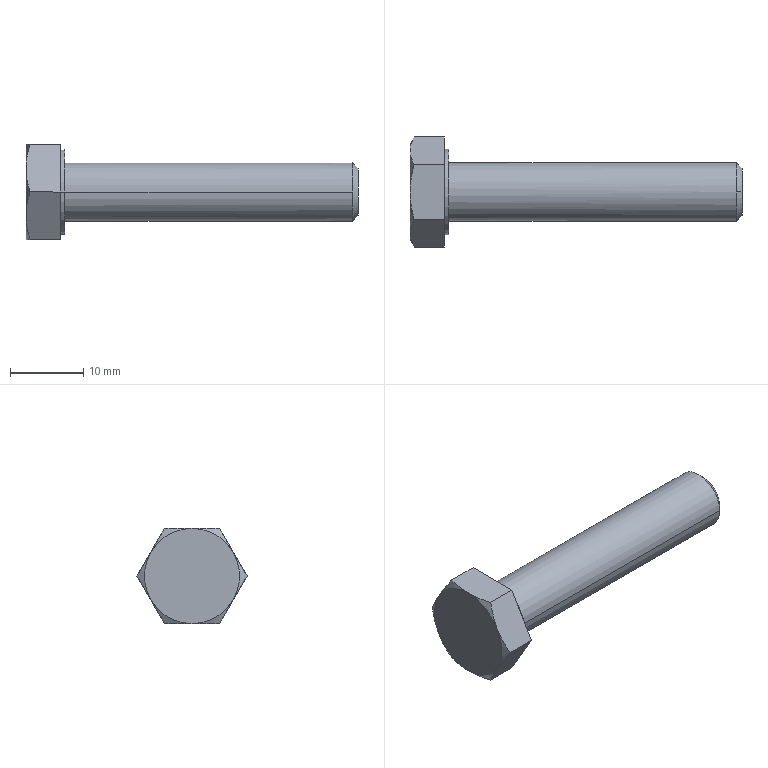Part | STEP file | 1 solid | 22 faces | box 45.3 x 15.011 x 13 mm | volume 2753 mm3 | plane 10 | cone 8 | cylinder 4 | commonest cylinder face diameters 8 x2 11.63 x2